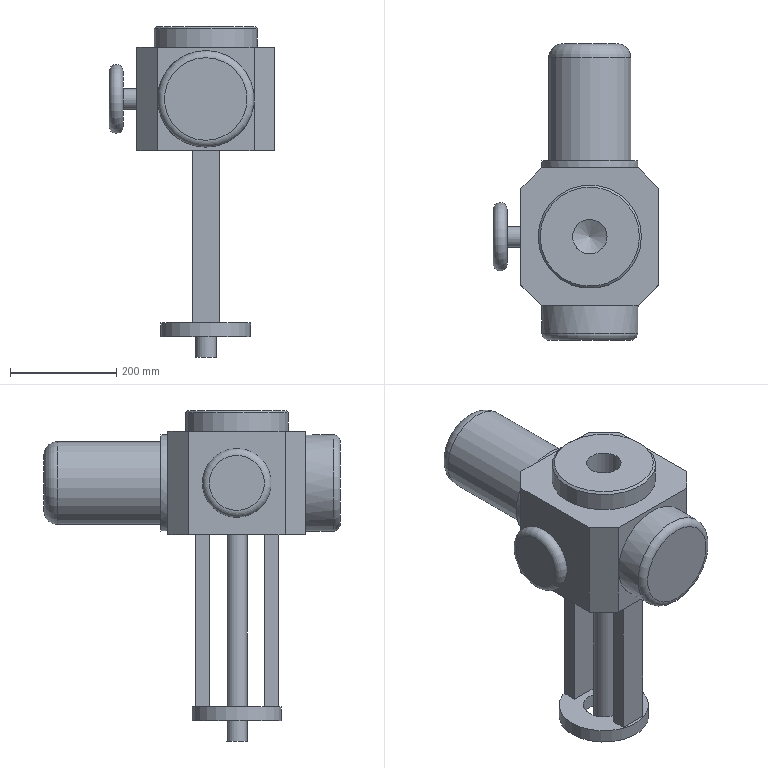Part | NX | features ABSOLUTE_DATUM_PLANE 3, ABSOLUTE_DATUM_AXIS 1, BREP 1 | 1 solid | 49 faces | box 312 x 559 x 624 mm | volume 21569285 mm3 | plane 31 | cylinder 11 | cone 4 | torus 3 | commonest cylinder face diameters 39 x2 182 x2 26 x1 52 x1 65 x1 78 x1
STEP:
#1=CARTESIAN_POINT('',(91.,-130.,578.5));
#2=VERTEX_POINT('',#1);
#3=CARTESIAN_POINT('',(-91.,-130.,578.5));
#4=VERTEX_POINT('',#3);
#5=CARTESIAN_POINT('',(0.,-130.,578.5));
#6=DIRECTION('',(0.,-1.,0.));
#7=DIRECTION('',(0.,0.,-1.));
#8=AXIS2_PLACEMENT_3D('',#5,#6,#7);
#9=CIRCLE('',#8,91.);
#10=EDGE_CURVE('',#2,#4,#9,.T.);
#11=ORIENTED_EDGE('',*,*,#10,.F.);
#12=CARTESIAN_POINT('',(91.,-130.,676.));
#13=VERTEX_POINT('',#12);
#14=CARTESIAN_POINT('',(91.,-130.,481.));
#15=DIRECTION('',(0.,0.,1.));
#16=VECTOR('',#15,1000.);
#17=LINE('',#14,#16);
#18=EDGE_CURVE('',#2,#13,#17,.T.);
#19=ORIENTED_EDGE('',*,*,#18,.T.);
#20=CARTESIAN_POINT('',(-91.,-130.,676.));
#21=VERTEX_POINT('',#20);
#22=CARTESIAN_POINT('',(-130.,-130.,676.));
#23=DIRECTION('',(1.,0.,0.));
#24=VECTOR('',#23,1000.);
#25=LINE('',#22,#24);
#26=EDGE_CURVE('',#21,#13,#25,.T.);
#27=ORIENTED_EDGE('',*,*,#26,.F.);
#28=CARTESIAN_POINT('',(-91.,-130.,481.));
#29=DIRECTION('',(0.,0.,-1.));
#30=VECTOR('',#29,1000.);
#31=LINE('',#28,#30);
#32=EDGE_CURVE('',#21,#4,#31,.T.);
#33=ORIENTED_EDGE('',*,*,#32,.T.);
#34=EDGE_LOOP('',(#11,#19,#27,#33));
#35=FACE_BOUND('',#34,.T.);
#36=CARTESIAN_POINT('',(130.,-130.,481.));
#37=DIRECTION('',(0.,-1.,0.));
#38=DIRECTION('',(0.,0.,-1.));
#39=AXIS2_PLACEMENT_3D('',#36,#37,#38);
#40=PLANE('',#39);
#41=ADVANCED_FACE('',(#35),#40,.T.);
#42=CARTESIAN_POINT('',(91.,130.,578.5));
#43=VERTEX_POINT('',#42);
#44=CARTESIAN_POINT('',(-91.,130.,578.5));
#45=VERTEX_POINT('',#44);
#46=CARTESIAN_POINT('',(0.,130.,578.5));
#47=DIRECTION('',(0.,1.,0.));
#48=DIRECTION('',(0.,0.,1.));
#49=AXIS2_PLACEMENT_3D('',#46,#47,#48);
#50=CIRCLE('',#49,91.);
#51=EDGE_CURVE('',#43,#45,#50,.T.);
#52=ORIENTED_EDGE('',*,*,#51,.F.);
#53=CARTESIAN_POINT('',(91.,130.,481.));
#54=VERTEX_POINT('',#53);
#55=CARTESIAN_POINT('',(91.,130.,481.));
#56=DIRECTION('',(0.,0.,-1.));
#57=VECTOR('',#56,1000.);
#58=LINE('',#55,#57);
#59=EDGE_CURVE('',#43,#54,#58,.T.);
#60=ORIENTED_EDGE('',*,*,#59,.T.);
#61=CARTESIAN_POINT('',(-91.,130.,481.));
#62=VERTEX_POINT('',#61);
#63=CARTESIAN_POINT('',(-130.,130.,481.));
#64=DIRECTION('',(1.,0.,0.));
#65=VECTOR('',#64,1000.);
#66=LINE('',#63,#65);
#67=EDGE_CURVE('',#62,#54,#66,.T.);
#68=ORIENTED_EDGE('',*,*,#67,.F.);
#69=CARTESIAN_POINT('',(-91.,130.,481.));
#70=DIRECTION('',(0.,0.,1.));
#71=VECTOR('',#70,1000.);
#72=LINE('',#69,#71);
#73=EDGE_CURVE('',#62,#45,#72,.T.);
#74=ORIENTED_EDGE('',*,*,#73,.T.);
#75=EDGE_LOOP('',(#52,#60,#68,#74));
#76=FACE_BOUND('',#75,.T.);
#77=CARTESIAN_POINT('',(-130.,130.,481.));
#78=DIRECTION('',(0.,1.,0.));
#79=DIRECTION('',(0.,0.,1.));
#80=AXIS2_PLACEMENT_3D('',#77,#78,#79);
#81=PLANE('',#80);
#82=ADVANCED_FACE('',(#76),#81,.T.);
#83=CARTESIAN_POINT('',(-26.,-78.,156.));
#84=VERTEX_POINT('',#83);
#85=CARTESIAN_POINT('',(-26.,-52.,156.));
#86=VERTEX_POINT('',#85);
#87=CARTESIAN_POINT('',(-26.,-78.,156.));
#88=DIRECTION('',(0.,1.,0.));
#89=VECTOR('',#88,1000.);
#90=LINE('',#87,#89);
#91=EDGE_CURVE('',#84,#86,#90,.T.);
#92=ORIENTED_EDGE('',*,*,#91,.T.);
#93=CARTESIAN_POINT('',(26.,-52.,156.));
#94=VERTEX_POINT('',#93);
#95=CARTESIAN_POINT('',(-26.,-52.,156.));
#96=DIRECTION('',(1.,0.,0.));
#97=VECTOR('',#96,1000.);
#98=LINE('',#95,#97);
#99=EDGE_CURVE('',#86,#94,#98,.T.);
#100=ORIENTED_EDGE('',*,*,#99,.T.);
#101=CARTESIAN_POINT('',(26.,-78.,156.));
#102=VERTEX_POINT('',#101);
#103=CARTESIAN_POINT('',(26.,-78.,156.));
#104=DIRECTION('',(0.,1.,0.));
#105=VECTOR('',#104,1000.);
#106=LINE('',#103,#105);
#107=EDGE_CURVE('',#102,#94,#106,.T.);
#108=ORIENTED_EDGE('',*,*,#107,.F.);
#109=CARTESIAN_POINT('',(-26.,-78.,156.));
#110=DIRECTION('',(1.,0.,0.));
#111=VECTOR('',#110,1000.);
#112=LINE('',#109,#111);
#113=EDGE_CURVE('',#84,#102,#112,.T.);
#114=ORIENTED_EDGE('',*,*,#113,.F.);
#115=EDGE_LOOP('',(#92,#100,#108,#114));
#116=FACE_BOUND('',#115,.T.);
#117=CARTESIAN_POINT('',(-26.,52.,156.));
#118=VERTEX_POINT('',#117);
#119=CARTESIAN_POINT('',(-26.,78.,156.));
#120=VERTEX_POINT('',#119);
#121=CARTESIAN_POINT('',(-26.,52.,156.));
#122=DIRECTION('',(0.,1.,0.));
#123=VECTOR('',#122,1000.);
#124=LINE('',#121,#123);
#125=EDGE_CURVE('',#118,#120,#124,.T.);
#126=ORIENTED_EDGE('',*,*,#125,.T.);
#127=CARTESIAN_POINT('',(26.,78.,156.));
#128=VERTEX_POINT('',#127);
#129=CARTESIAN_POINT('',(-26.,78.,156.));
#130=DIRECTION('',(1.,0.,0.));
#131=VECTOR('',#130,1000.);
#132=LINE('',#129,#131);
#133=EDGE_CURVE('',#120,#128,#132,.T.);
#134=ORIENTED_EDGE('',*,*,#133,.T.);
#135=CARTESIAN_POINT('',(26.,52.,156.));
#136=VERTEX_POINT('',#135);
#137=CARTESIAN_POINT('',(26.,52.,156.));
#138=DIRECTION('',(0.,1.,0.));
#139=VECTOR('',#138,1000.);
#140=LINE('',#137,#139);
#141=EDGE_CURVE('',#136,#128,#140,.T.);
#142=ORIENTED_EDGE('',*,*,#141,.F.);
#143=CARTESIAN_POINT('',(-26.,52.,156.));
#144=DIRECTION('',(1.,0.,0.));
#145=VECTOR('',#144,1000.);
#146=LINE('',#143,#145);
#147=EDGE_CURVE('',#118,#136,#146,.T.);
#148=ORIENTED_EDGE('',*,*,#147,.F.);
#149=EDGE_LOOP('',(#126,#134,#142,#148));
#150=FACE_BOUND('',#149,.T.);
#151=CARTESIAN_POINT('',(39.,0.,156.));
#152=VERTEX_POINT('',#151);
#153=CARTESIAN_POINT('',(0.,0.,156.));
#154=DIRECTION('',(0.,0.,1.));
#155=DIRECTION('',(1.,0.,0.));
#156=AXIS2_PLACEMENT_3D('',#153,#154,#155);
#157=CIRCLE('',#156,39.);
#158=EDGE_CURVE('',#152,#152,#157,.F.);
#159=ORIENTED_EDGE('',*,*,#158,.T.);
#160=EDGE_LOOP('',(#159));
#161=FACE_BOUND('',#160,.T.);
#162=CARTESIAN_POINT('',(-84.5,0.,156.));
#163=VERTEX_POINT('',#162);
#164=CARTESIAN_POINT('',(0.,0.,156.));
#165=DIRECTION('',(0.,0.,-1.));
#166=DIRECTION('',(-1.,0.,0.));
#167=AXIS2_PLACEMENT_3D('',#164,#165,#166);
#168=CIRCLE('',#167,84.5);
#169=EDGE_CURVE('',#163,#163,#168,.T.);
#170=ORIENTED_EDGE('',*,*,#169,.F.);
#171=EDGE_LOOP('',(#170));
#172=FACE_BOUND('',#171,.T.);
#173=CARTESIAN_POINT('',(0.,0.,156.));
#174=DIRECTION('',(0.,0.,1.));
#175=DIRECTION('',(1.,0.,0.));
#176=AXIS2_PLACEMENT_3D('',#173,#174,#175);
#177=PLANE('',#176);
#178=ADVANCED_FACE('',(#116,#150,#161,#172),#177,.T.);
#179=CARTESIAN_POINT('',(39.,0.,130.));
#180=VERTEX_POINT('',#179);
#181=CARTESIAN_POINT('',(0.,0.,130.));
#182=DIRECTION('',(0.,0.,1.));
#183=DIRECTION('',(1.,0.,0.));
#184=AXIS2_PLACEMENT_3D('',#181,#182,#183);
#185=CIRCLE('',#184,39.);
#186=EDGE_CURVE('',#180,#180,#185,.T.);
#187=ORIENTED_EDGE('',*,*,#186,.T.);
#188=EDGE_LOOP('',(#187));
#189=FACE_BOUND('',#188,.T.);
#190=CARTESIAN_POINT('',(84.5,0.,130.));
#191=VERTEX_POINT('',#190);
#192=CARTESIAN_POINT('',(0.,0.,130.));
#193=DIRECTION('',(0.,0.,1.));
#194=DIRECTION('',(1.,0.,0.));
#195=AXIS2_PLACEMENT_3D('',#192,#193,#194);
#196=CIRCLE('',#195,84.5);
#197=EDGE_CURVE('',#191,#191,#196,.T.);
#198=ORIENTED_EDGE('',*,*,#197,.F.);
#199=EDGE_LOOP('',(#198));
#200=FACE_BOUND('',#199,.T.);
#201=CARTESIAN_POINT('',(0.,0.,130.));
#202=DIRECTION('',(0.,0.,-1.));
#203=DIRECTION('',(-1.,0.,0.));
#204=AXIS2_PLACEMENT_3D('',#201,#202,#203);
#205=PLANE('',#204);
#206=ADVANCED_FACE('',(#189,#200),#205,.T.);
#207=ORIENTED_EDGE('',*,*,#169,.T.);
#208=EDGE_LOOP('',(#207));
#209=FACE_BOUND('',#208,.T.);
#210=ORIENTED_EDGE('',*,*,#197,.T.);
#211=EDGE_LOOP('',(#210));
#212=FACE_BOUND('',#211,.T.);
#213=CARTESIAN_POINT('',(0.,0.,130.));
#214=DIRECTION('',(0.,0.,1.));
#215=DIRECTION('',(1.,0.,0.));
#216=AXIS2_PLACEMENT_3D('',#213,#214,#215);
#217=CYLINDRICAL_SURFACE('',#216,84.5);
#218=ADVANCED_FACE('',(#209,#212),#217,.T.);
#219=ORIENTED_EDGE('',*,*,#158,.F.);
#220=EDGE_LOOP('',(#219));
#221=FACE_BOUND('',#220,.T.);
#222=ORIENTED_EDGE('',*,*,#186,.F.);
#223=EDGE_LOOP('',(#222));
#224=FACE_BOUND('',#223,.T.);
#225=CARTESIAN_POINT('',(0.,0.,130.));
#226=DIRECTION('',(0.,0.,1.));
#227=DIRECTION('',(1.,0.,0.));
#228=AXIS2_PLACEMENT_3D('',#225,#226,#227);
#229=CYLINDRICAL_SURFACE('',#228,39.);
#230=ADVANCED_FACE('',(#221,#224),#229,.F.);
#231=ORIENTED_EDGE('',*,*,#125,.F.);
#232=CARTESIAN_POINT('',(-26.,52.,481.));
#233=VERTEX_POINT('',#232);
#234=CARTESIAN_POINT('',(-26.,52.,481.));
#235=DIRECTION('',(0.,0.,1.));
#236=VECTOR('',#235,1000.);
#237=LINE('',#234,#236);
#238=EDGE_CURVE('',#118,#233,#237,.T.);
#239=ORIENTED_EDGE('',*,*,#238,.T.);
#240=CARTESIAN_POINT('',(-26.,78.,481.));
#241=VERTEX_POINT('',#240);
#242=CARTESIAN_POINT('',(-26.,52.,481.));
#243=DIRECTION('',(0.,1.,0.));
#244=VECTOR('',#243,1000.);
#245=LINE('',#242,#244);
#246=EDGE_CURVE('',#233,#241,#245,.T.);
#247=ORIENTED_EDGE('',*,*,#246,.T.);
#248=CARTESIAN_POINT('',(-26.,78.,481.));
#249=DIRECTION('',(0.,0.,1.));
#250=VECTOR('',#249,1000.);
#251=LINE('',#248,#250);
#252=EDGE_CURVE('',#120,#241,#251,.T.);
#253=ORIENTED_EDGE('',*,*,#252,.F.);
#254=EDGE_LOOP('',(#231,#239,#247,#253));
#255=FACE_BOUND('',#254,.T.);
#256=CARTESIAN_POINT('',(-26.,52.,156.));
#257=DIRECTION('',(-1.,0.,0.));
#258=DIRECTION('',(0.,0.,1.));
#259=AXIS2_PLACEMENT_3D('',#256,#257,#258);
#260=PLANE('',#259);
#261=ADVANCED_FACE('',(#255),#260,.T.);
#262=ORIENTED_EDGE('',*,*,#133,.F.);
#263=ORIENTED_EDGE('',*,*,#252,.T.);
#264=CARTESIAN_POINT('',(26.,78.,481.));
#265=VERTEX_POINT('',#264);
#266=CARTESIAN_POINT('',(-26.,78.,481.));
#267=DIRECTION('',(1.,0.,0.));
#268=VECTOR('',#267,1000.);
#269=LINE('',#266,#268);
#270=EDGE_CURVE('',#241,#265,#269,.T.);
#271=ORIENTED_EDGE('',*,*,#270,.T.);
#272=CARTESIAN_POINT('',(26.,78.,481.));
#273=DIRECTION('',(0.,0.,1.));
#274=VECTOR('',#273,1000.);
#275=LINE('',#272,#274);
#276=EDGE_CURVE('',#128,#265,#275,.T.);
#277=ORIENTED_EDGE('',*,*,#276,.F.);
#278=EDGE_LOOP('',(#262,#263,#271,#277));
#279=FACE_BOUND('',#278,.T.);
#280=CARTESIAN_POINT('',(-26.,78.,156.));
#281=DIRECTION('',(0.,1.,0.));
#282=DIRECTION('',(0.,0.,1.));
#283=AXIS2_PLACEMENT_3D('',#280,#281,#282);
#284=PLANE('',#283);
#285=ADVANCED_FACE('',(#279),#284,.T.);
#286=ORIENTED_EDGE('',*,*,#141,.T.);
#287=ORIENTED_EDGE('',*,*,#276,.T.);
#288=CARTESIAN_POINT('',(26.,52.,481.));
#289=VERTEX_POINT('',#288);
#290=CARTESIAN_POINT('',(26.,52.,481.));
#291=DIRECTION('',(0.,1.,0.));
#292=VECTOR('',#291,1000.);
#293=LINE('',#290,#292);
#294=EDGE_CURVE('',#289,#265,#293,.T.);
#295=ORIENTED_EDGE('',*,*,#294,.F.);
#296=CARTESIAN_POINT('',(26.,52.,481.));
#297=DIRECTION('',(0.,0.,1.));
#298=VECTOR('',#297,1000.);
#299=LINE('',#296,#298);
#300=EDGE_CURVE('',#136,#289,#299,.T.);
#301=ORIENTED_EDGE('',*,*,#300,.F.);
#302=EDGE_LOOP('',(#286,#287,#295,#301));
#303=FACE_BOUND('',#302,.T.);
#304=CARTESIAN_POINT('',(26.,78.,156.));
#305=DIRECTION('',(1.,0.,0.));
#306=DIRECTION('',(0.,0.,-1.));
#307=AXIS2_PLACEMENT_3D('',#304,#305,#306);
#308=PLANE('',#307);
#309=ADVANCED_FACE('',(#303),#308,.T.);
#310=ORIENTED_EDGE('',*,*,#238,.F.);
#311=ORIENTED_EDGE('',*,*,#147,.T.);
#312=ORIENTED_EDGE('',*,*,#300,.T.);
#313=CARTESIAN_POINT('',(-26.,52.,481.));
#314=DIRECTION('',(1.,0.,0.));
#315=VECTOR('',#314,1000.);
#316=LINE('',#313,#315);
#317=EDGE_CURVE('',#233,#289,#316,.T.);
#318=ORIENTED_EDGE('',*,*,#317,.F.);
#319=EDGE_LOOP('',(#310,#311,#312,#318));
#320=FACE_BOUND('',#319,.T.);
#321=CARTESIAN_POINT('',(26.,52.,156.));
#322=DIRECTION('',(0.,-1.,0.));
#323=DIRECTION('',(0.,0.,-1.));
#324=AXIS2_PLACEMENT_3D('',#321,#322,#323);
#325=PLANE('',#324);
#326=ADVANCED_FACE('',(#320),#325,.T.);
#327=ORIENTED_EDGE('',*,*,#91,.F.);
#328=CARTESIAN_POINT('',(-26.,-78.,481.));
#329=VERTEX_POINT('',#328);
#330=CARTESIAN_POINT('',(-26.,-78.,481.));
#331=DIRECTION('',(0.,0.,1.));
#332=VECTOR('',#331,1000.);
#333=LINE('',#330,#332);
#334=EDGE_CURVE('',#84,#329,#333,.T.);
#335=ORIENTED_EDGE('',*,*,#334,.T.);
#336=CARTESIAN_POINT('',(-26.,-52.,481.));
#337=VERTEX_POINT('',#336);
#338=CARTESIAN_POINT('',(-26.,-78.,481.));
#339=DIRECTION('',(0.,1.,0.));
#340=VECTOR('',#339,1000.);
#341=LINE('',#338,#340);
#342=EDGE_CURVE('',#329,#337,#341,.T.);
#343=ORIENTED_EDGE('',*,*,#342,.T.);
#344=CARTESIAN_POINT('',(-26.,-52.,481.));
#345=DIRECTION('',(0.,0.,1.));
#346=VECTOR('',#345,1000.);
#347=LINE('',#344,#346);
#348=EDGE_CURVE('',#86,#337,#347,.T.);
#349=ORIENTED_EDGE('',*,*,#348,.F.);
#350=EDGE_LOOP('',(#327,#335,#343,#349));
#351=FACE_BOUND('',#350,.T.);
#352=CARTESIAN_POINT('',(-26.,-78.,156.));
#353=DIRECTION('',(-1.,0.,0.));
#354=DIRECTION('',(0.,0.,1.));
#355=AXIS2_PLACEMENT_3D('',#352,#353,#354);
#356=PLANE('',#355);
#357=ADVANCED_FACE('',(#351),#356,.T.);
#358=ORIENTED_EDGE('',*,*,#99,.F.);
#359=ORIENTED_EDGE('',*,*,#348,.T.);
#360=CARTESIAN_POINT('',(26.,-52.,481.));
#361=VERTEX_POINT('',#360);
#362=CARTESIAN_POINT('',(-26.,-52.,481.));
#363=DIRECTION('',(1.,0.,0.));
#364=VECTOR('',#363,1000.);
#365=LINE('',#362,#364);
#366=EDGE_CURVE('',#337,#361,#365,.T.);
#367=ORIENTED_EDGE('',*,*,#366,.T.);
#368=CARTESIAN_POINT('',(26.,-52.,481.));
#369=DIRECTION('',(0.,0.,1.));
#370=VECTOR('',#369,1000.);
#371=LINE('',#368,#370);
#372=EDGE_CURVE('',#94,#361,#371,.T.);
#373=ORIENTED_EDGE('',*,*,#372,.F.);
#374=EDGE_LOOP('',(#358,#359,#367,#373));
#375=FACE_BOUND('',#374,.T.);
#376=CARTESIAN_POINT('',(-26.,-52.,156.));
#377=DIRECTION('',(0.,1.,0.));
#378=DIRECTION('',(0.,0.,1.));
#379=AXIS2_PLACEMENT_3D('',#376,#377,#378);
#380=PLANE('',#379);
#381=ADVANCED_FACE('',(#375),#380,.T.);
#382=ORIENTED_EDGE('',*,*,#107,.T.);
#383=ORIENTED_EDGE('',*,*,#372,.T.);
#384=CARTESIAN_POINT('',(26.,-78.,481.));
#385=VERTEX_POINT('',#384);
#386=CARTESIAN_POINT('',(26.,-78.,481.));
#387=DIRECTION('',(0.,1.,0.));
#388=VECTOR('',#387,1000.);
#389=LINE('',#386,#388);
#390=EDGE_CURVE('',#385,#361,#389,.T.);
#391=ORIENTED_EDGE('',*,*,#390,.F.);
#392=CARTESIAN_POINT('',(26.,-78.,481.));
#393=DIRECTION('',(0.,0.,1.));
#394=VECTOR('',#393,1000.);
#395=LINE('',#392,#394);
#396=EDGE_CURVE('',#102,#385,#395,.T.);
#397=ORIENTED_EDGE('',*,*,#396,.F.);
#398=EDGE_LOOP('',(#382,#383,#391,#397));
#399=FACE_BOUND('',#398,.T.);
#400=CARTESIAN_POINT('',(26.,-52.,156.));
#401=DIRECTION('',(1.,0.,0.));
#402=DIRECTION('',(0.,0.,-1.));
#403=AXIS2_PLACEMENT_3D('',#400,#401,#402);
#404=PLANE('',#403);
#405=ADVANCED_FACE('',(#399),#404,.T.);
#406=ORIENTED_EDGE('',*,*,#334,.F.);
#407=ORIENTED_EDGE('',*,*,#113,.T.);
#408=ORIENTED_EDGE('',*,*,#396,.T.);
#409=CARTESIAN_POINT('',(-26.,-78.,481.));
#410=DIRECTION('',(1.,0.,0.));
#411=VECTOR('',#410,1000.);
#412=LINE('',#409,#411);
#413=EDGE_CURVE('',#329,#385,#412,.T.);
#414=ORIENTED_EDGE('',*,*,#413,.F.);
#415=EDGE_LOOP('',(#406,#407,#408,#414));
#416=FACE_BOUND('',#415,.T.);
#417=CARTESIAN_POINT('',(26.,-78.,156.));
#418=DIRECTION('',(0.,-1.,0.));
#419=DIRECTION('',(0.,0.,-1.));
#420=AXIS2_PLACEMENT_3D('',#417,#418,#419);
#421=PLANE('',#420);
#422=ADVANCED_FACE('',(#416),#421,.T.);
#423=CARTESIAN_POINT('',(-130.,0.,598.));
#424=VERTEX_POINT('',#423);
#425=CARTESIAN_POINT('',(-130.,0.,578.5));
#426=DIRECTION('',(-1.,0.,0.));
#427=DIRECTION('',(0.,0.,1.));
#428=AXIS2_PLACEMENT_3D('',#425,#426,#427);
#429=CIRCLE('',#428,19.5);
#430=EDGE_CURVE('',#424,#424,#429,.T.);
#431=ORIENTED_EDGE('',*,*,#430,.F.);
#432=EDGE_LOOP('',(#431));
#433=FACE_BOUND('',#432,.T.);
#434=CARTESIAN_POINT('',(-130.,-91.,676.));
#435=VERTEX_POINT('',#434);
#436=CARTESIAN_POINT('',(-130.,91.,676.));
#437=VERTEX_POINT('',#436);
#438=CARTESIAN_POINT('',(-130.,-130.,676.));
#439=DIRECTION('',(0.,1.,0.));
#440=VECTOR('',#439,1000.);
#441=LINE('',#438,#440);
#442=EDGE_CURVE('',#435,#437,#441,.T.);
#443=ORIENTED_EDGE('',*,*,#442,.T.);
#444=CARTESIAN_POINT('',(-130.,91.,481.));
#445=VERTEX_POINT('',#444);
#446=CARTESIAN_POINT('',(-130.,91.,481.));
#447=DIRECTION('',(0.,0.,-1.));
#448=VECTOR('',#447,1000.);
#449=LINE('',#446,#448);
#450=EDGE_CURVE('',#437,#445,#449,.T.);
#451=ORIENTED_EDGE('',*,*,#450,.T.);
#452=CARTESIAN_POINT('',(-130.,-91.,481.));
#453=VERTEX_POINT('',#452);
#454=CARTESIAN_POINT('',(-130.,-130.,481.));
#455=DIRECTION('',(0.,1.,0.));
#456=VECTOR('',#455,1000.);
#457=LINE('',#454,#456);
#458=EDGE_CURVE('',#453,#445,#457,.T.);
#459=ORIENTED_EDGE('',*,*,#458,.F.);
#460=CARTESIAN_POINT('',(-130.,-91.,481.));
#461=DIRECTION('',(0.,0.,1.));
#462=VECTOR('',#461,1000.);
#463=LINE('',#460,#462);
#464=EDGE_CURVE('',#453,#435,#463,.T.);
#465=ORIENTED_EDGE('',*,*,#464,.T.);
#466=EDGE_LOOP('',(#443,#451,#459,#465));
#467=FACE_BOUND('',#466,.T.);
#468=CARTESIAN_POINT('',(-130.,-130.,481.));
#469=DIRECTION('',(-1.,0.,0.));
#470=DIRECTION('',(0.,0.,1.));
#471=AXIS2_PLACEMENT_3D('',#468,#469,#470);
#472=PLANE('',#471);
#473=ADVANCED_FACE('',(#433,#467),#472,.T.);
#474=CARTESIAN_POINT('',(0.,130.,578.5));
#475=DIRECTION('',(0.,1.,0.));
#476=DIRECTION('',(0.,0.,1.));
#477=AXIS2_PLACEMENT_3D('',#474,#475,#476);
#478=CIRCLE('',#477,91.);
#479=EDGE_CURVE('',#45,#43,#478,.T.);
#480=ORIENTED_EDGE('',*,*,#479,.F.);
#481=CARTESIAN_POINT('',(-91.,130.,676.));
#482=VERTEX_POINT('',#481);
#483=CARTESIAN_POINT('',(-91.,130.,481.));
#484=DIRECTION('',(0.,0.,1.));
#485=VECTOR('',#484,1000.);
#486=LINE('',#483,#485);
#487=EDGE_CURVE('',#45,#482,#486,.T.);
#488=ORIENTED_EDGE('',*,*,#487,.T.);
#489=CARTESIAN_POINT('',(91.,130.,676.));
#490=VERTEX_POINT('',#489);
#491=CARTESIAN_POINT('',(-130.,130.,676.));
#492=DIRECTION('',(1.,0.,0.));
#493=VECTOR('',#492,1000.);
#494=LINE('',#491,#493);
#495=EDGE_CURVE('',#482,#490,#494,.T.);
#496=ORIENTED_EDGE('',*,*,#495,.T.);
#497=CARTESIAN_POINT('',(91.,130.,481.));
#498=DIRECTION('',(0.,0.,-1.));
#499=VECTOR('',#498,1000.);
#500=LINE('',#497,#499);
#501=EDGE_CURVE('',#490,#43,#500,.T.);
#502=ORIENTED_EDGE('',*,*,#501,.T.);
#503=EDGE_LOOP('',(#480,#488,#496,#502));
#504=FACE_BOUND('',#503,.T.);
#505=CARTESIAN_POINT('',(-130.,130.,481.));
#506=DIRECTION('',(0.,1.,0.));
#507=DIRECTION('',(0.,0.,1.));
#508=AXIS2_PLACEMENT_3D('',#505,#506,#507);
#509=PLANE('',#508);
#510=ADVANCED_FACE('',(#504),#509,.T.);
#511=CARTESIAN_POINT('',(130.,-91.,481.));
#512=VERTEX_POINT('',#511);
#513=CARTESIAN_POINT('',(130.,91.,481.));
#514=VERTEX_POINT('',#513);
#515=CARTESIAN_POINT('',(130.,-130.,481.));
#516=DIRECTION('',(0.,1.,0.));
#517=VECTOR('',#516,1000.);
#518=LINE('',#515,#517);
#519=EDGE_CURVE('',#512,#514,#518,.T.);
#520=ORIENTED_EDGE('',*,*,#519,.T.);
#521=CARTESIAN_POINT('',(130.,91.,676.));
#522=VERTEX_POINT('',#521);
#523=CARTESIAN_POINT('',(130.,91.,481.));
#524=DIRECTION('',(0.,0.,1.));
#525=VECTOR('',#524,1000.);
#526=LINE('',#523,#525);
#527=EDGE_CURVE('',#514,#522,#526,.T.);
#528=ORIENTED_EDGE('',*,*,#527,.T.);
#529=CARTESIAN_POINT('',(130.,-91.,676.));
#530=VERTEX_POINT('',#529);
#531=CARTESIAN_POINT('',(130.,-130.,676.));
#532=DIRECTION('',(0.,1.,0.));
#533=VECTOR('',#532,1000.);
#534=LINE('',#531,#533);
#535=EDGE_CURVE('',#530,#522,#534,.T.);
#536=ORIENTED_EDGE('',*,*,#535,.F.);
#537=CARTESIAN_POINT('',(130.,-91.,481.));
#538=DIRECTION('',(0.,0.,-1.));
#539=VECTOR('',#538,1000.);
#540=LINE('',#537,#539);
#541=EDGE_CURVE('',#530,#512,#540,.T.);
#542=ORIENTED_EDGE('',*,*,#541,.T.);
#543=EDGE_LOOP('',(#520,#528,#536,#542));
#544=FACE_BOUND('',#543,.T.);
#545=CARTESIAN_POINT('',(130.,130.,481.));
#546=DIRECTION('',(1.,0.,0.));
#547=DIRECTION('',(0.,0.,-1.));
#548=AXIS2_PLACEMENT_3D('',#545,#546,#547);
#549=PLANE('',#548);
#550=ADVANCED_FACE('',(#544),#549,.T.);
#551=CARTESIAN_POINT('',(-19.5,0.,481.));
#552=VERTEX_POINT('',#551);
#553=CARTESIAN_POINT('',(0.,0.,481.));
#554=DIRECTION('',(0.,0.,-1.));
#555=DIRECTION('',(-1.,0.,0.));
#556=AXIS2_PLACEMENT_3D('',#553,#554,#555);
#557=CIRCLE('',#556,19.5);
#558=EDGE_CURVE('',#552,#552,#557,.T.);
#559=ORIENTED_EDGE('',*,*,#558,.F.);
#560=EDGE_LOOP('',(#559));
#561=FACE_BOUND('',#560,.T.);
#562=ORIENTED_EDGE('',*,*,#270,.F.);
#563=ORIENTED_EDGE('',*,*,#246,.F.);
#564=ORIENTED_EDGE('',*,*,#317,.T.);
#565=ORIENTED_EDGE('',*,*,#294,.T.);
#566=EDGE_LOOP('',(#562,#563,#564,#565));
#567=FACE_BOUND('',#566,.T.);
#568=ORIENTED_EDGE('',*,*,#366,.F.);
#569=ORIENTED_EDGE('',*,*,#342,.F.);
#570=ORIENTED_EDGE('',*,*,#413,.T.);
#571=ORIENTED_EDGE('',*,*,#390,.T.);
#572=EDGE_LOOP('',(#568,#569,#570,#571));
#573=FACE_BOUND('',#572,.T.);
#574=ORIENTED_EDGE('',*,*,#67,.T.);
#575=CARTESIAN_POINT('',(240.5,-19.5,481.));
#576=DIRECTION('',(-0.7071,0.7071,0.));
#577=VECTOR('',#576,1000.);
#578=LINE('',#575,#577);
#579=EDGE_CURVE('',#54,#514,#578,.F.);
#580=ORIENTED_EDGE('',*,*,#579,.T.);
#581=ORIENTED_EDGE('',*,*,#519,.F.);
#582=CARTESIAN_POINT('',(91.,-130.,481.));
#583=VERTEX_POINT('',#582);
#584=CARTESIAN_POINT('',(110.5,-110.5,481.));
#585=DIRECTION('',(0.7071,0.7071,0.));
#586=VECTOR('',#585,1000.);
#587=LINE('',#584,#586);
#588=EDGE_CURVE('',#512,#583,#587,.F.);
#589=ORIENTED_EDGE('',*,*,#588,.T.);
#590=CARTESIAN_POINT('',(-91.,-130.,481.));
#591=VERTEX_POINT('',#590);
#592=CARTESIAN_POINT('',(-130.,-130.,481.));
#593=DIRECTION('',(1.,0.,0.));
#594=VECTOR('',#593,1000.);
#595=LINE('',#592,#594);
#596=EDGE_CURVE('',#591,#583,#595,.T.);
#597=ORIENTED_EDGE('',*,*,#596,.F.);
#598=CARTESIAN_POINT('',(19.5,-240.5,481.));
#599=DIRECTION('',(0.7071,-0.7071,0.));
#600=VECTOR('',#599,1000.);
#601=LINE('',#598,#600);
#602=EDGE_CURVE('',#591,#453,#601,.F.);
#603=ORIENTED_EDGE('',*,*,#602,.T.);
#604=ORIENTED_EDGE('',*,*,#458,.T.);
#605=CARTESIAN_POINT('',(-110.5,110.5,481.));
#606=DIRECTION('',(-0.7071,-0.7071,0.));
#607=VECTOR('',#606,1000.);
#608=LINE('',#605,#607);
#609=EDGE_CURVE('',#445,#62,#608,.F.);
#610=ORIENTED_EDGE('',*,*,#609,.T.);
#611=EDGE_LOOP('',(#574,#580,#581,#589,#597,#603,#604,#610));
#612=FACE_BOUND('',#611,.T.);
#613=CARTESIAN_POINT('',(130.,-130.,481.));
#614=DIRECTION('',(0.,0.,-1.));
#615=DIRECTION('',(-1.,0.,0.));
#616=AXIS2_PLACEMENT_3D('',#613,#614,#615);
#617=PLANE('',#616);
#618=ADVANCED_FACE('',(#561,#567,#573,#612),#617,.T.);
#619=CARTESIAN_POINT('',(0.,-130.,578.5));
#620=DIRECTION('',(0.,-1.,0.));
#621=DIRECTION('',(0.,0.,-1.));
#622=AXIS2_PLACEMENT_3D('',#619,#620,#621);
#623=CIRCLE('',#622,91.);
#624=EDGE_CURVE('',#4,#2,#623,.T.);
#625=ORIENTED_EDGE('',*,*,#624,.F.);
#626=CARTESIAN_POINT('',(-91.,-130.,481.));
#627=DIRECTION('',(0.,0.,-1.));
#628=VECTOR('',#627,1000.);
#629=LINE('',#626,#628);
#630=EDGE_CURVE('',#4,#591,#629,.T.);
#631=ORIENTED_EDGE('',*,*,#630,.T.);
#632=ORIENTED_EDGE('',*,*,#596,.T.);
#633=CARTESIAN_POINT('',(91.,-130.,481.));
#634=DIRECTION('',(0.,0.,1.));
#635=VECTOR('',#634,1000.);
#636=LINE('',#633,#635);
#637=EDGE_CURVE('',#583,#2,#636,.T.);
#638=ORIENTED_EDGE('',*,*,#637,.T.);
#639=EDGE_LOOP('',(#625,#631,#632,#638));
#640=FACE_BOUND('',#639,.T.);
#641=CARTESIAN_POINT('',(130.,-130.,481.));
#642=DIRECTION('',(0.,-1.,0.));
#643=DIRECTION('',(0.,0.,-1.));
#644=AXIS2_PLACEMENT_3D('',#641,#642,#643);
#645=PLANE('',#644);
#646=ADVANCED_FACE('',(#640),#645,.T.);
#647=CARTESIAN_POINT('',(97.5,0.,676.));
#648=VERTEX_POINT('',#647);
#649=CARTESIAN_POINT('',(0.,0.,676.));
#650=DIRECTION('',(0.,0.,1.));
#651=DIRECTION('',(1.,0.,0.));
#652=AXIS2_PLACEMENT_3D('',#649,#650,#651);
#653=CIRCLE('',#652,97.5);
#654=EDGE_CURVE('',#648,#648,#653,.T.);
#655=ORIENTED_EDGE('',*,*,#654,.F.);
#656=EDGE_LOOP('',(#655));
#657=FACE_BOUND('',#656,.T.);
#658=ORIENTED_EDGE('',*,*,#535,.T.);
#659=CARTESIAN_POINT('',(110.5,110.5,676.));
#660=DIRECTION('',(0.7071,-0.7071,0.));
#661=VECTOR('',#660,1000.);
#662=LINE('',#659,#661);
#663=EDGE_CURVE('',#522,#490,#662,.F.);
#664=ORIENTED_EDGE('',*,*,#663,.T.);
#665=ORIENTED_EDGE('',*,*,#495,.F.);
#666=CARTESIAN_POINT('',(-240.5,-19.5,676.));
#667=DIRECTION('',(0.7071,0.7071,0.));
#668=VECTOR('',#667,1000.);
#669=LINE('',#666,#668);
#670=EDGE_CURVE('',#482,#437,#669,.F.);
#671=ORIENTED_EDGE('',*,*,#670,.T.);
#672=ORIENTED_EDGE('',*,*,#442,.F.);
#673=CARTESIAN_POINT('',(-110.5,-110.5,676.));
#674=DIRECTION('',(-0.7071,0.7071,0.));
#675=VECTOR('',#674,1000.);
#676=LINE('',#673,#675);
#677=EDGE_CURVE('',#435,#21,#676,.F.);
#678=ORIENTED_EDGE('',*,*,#677,.T.);
#679=ORIENTED_EDGE('',*,*,#26,.T.);
#680=CARTESIAN_POINT('',(-19.5,-240.5,676.));
#681=DIRECTION('',(-0.7071,-0.7071,0.));
#682=VECTOR('',#681,1000.);
#683=LINE('',#680,#682);
#684=EDGE_CURVE('',#13,#530,#683,.F.);
#685=ORIENTED_EDGE('',*,*,#684,.T.);
#686=EDGE_LOOP('',(#658,#664,#665,#671,#672,#678,#679,#685));
#687=FACE_BOUND('',#686,.T.);
#688=CARTESIAN_POINT('',(-130.,-130.,676.));
#689=DIRECTION('',(0.,0.,1.));
#690=DIRECTION('',(1.,0.,0.));
#691=AXIS2_PLACEMENT_3D('',#688,#689,#690);
#692=PLANE('',#691);
#693=ADVANCED_FACE('',(#657,#687),#692,.T.);
#694=ORIENTED_EDGE('',*,*,#579,.F.);
#695=ORIENTED_EDGE('',*,*,#59,.F.);
#696=ORIENTED_EDGE('',*,*,#501,.F.);
#697=ORIENTED_EDGE('',*,*,#663,.F.);
#698=ORIENTED_EDGE('',*,*,#527,.F.);
#699=EDGE_LOOP('',(#694,#695,#696,#697,#698));
#700=FACE_BOUND('',#699,.T.);
#701=CARTESIAN_POINT('',(130.,91.,481.));
#702=DIRECTION('',(-0.7071,-0.7071,0.));
#703=DIRECTION('',(0.7071,-0.7071,0.));
#704=AXIS2_PLACEMENT_3D('',#701,#702,#703);
#705=PLANE('',#704);
#706=ADVANCED_FACE('',(#700),#705,.F.);
#707=ORIENTED_EDGE('',*,*,#609,.F.);
#708=ORIENTED_EDGE('',*,*,#450,.F.);
#709=ORIENTED_EDGE('',*,*,#670,.F.);
#710=ORIENTED_EDGE('',*,*,#487,.F.);
#711=ORIENTED_EDGE('',*,*,#73,.F.);
#712=EDGE_LOOP('',(#707,#708,#709,#710,#711));
#713=FACE_BOUND('',#712,.T.);
#714=CARTESIAN_POINT('',(-91.,130.,481.));
#715=DIRECTION('',(0.7071,-0.7071,0.));
#716=DIRECTION('',(0.7071,0.7071,0.));
#717=AXIS2_PLACEMENT_3D('',#714,#715,#716);
#718=PLANE('',#717);
#719=ADVANCED_FACE('',(#713),#718,.F.);
#720=ORIENTED_EDGE('',*,*,#588,.F.);
#721=ORIENTED_EDGE('',*,*,#541,.F.);
#722=ORIENTED_EDGE('',*,*,#684,.F.);
#723=ORIENTED_EDGE('',*,*,#18,.F.);
#724=ORIENTED_EDGE('',*,*,#637,.F.);
#725=EDGE_LOOP('',(#720,#721,#722,#723,#724));
#726=FACE_BOUND('',#725,.T.);
#727=CARTESIAN_POINT('',(91.,-130.,481.));
#728=DIRECTION('',(-0.7071,0.7071,0.));
#729=DIRECTION('',(-0.7071,-0.7071,0.));
#730=AXIS2_PLACEMENT_3D('',#727,#728,#729);
#731=PLANE('',#730);
#732=ADVANCED_FACE('',(#726),#731,.F.);
#733=ORIENTED_EDGE('',*,*,#602,.F.);
#734=ORIENTED_EDGE('',*,*,#630,.F.);
#735=ORIENTED_EDGE('',*,*,#32,.F.);
#736=ORIENTED_EDGE('',*,*,#677,.F.);
#737=ORIENTED_EDGE('',*,*,#464,.F.);
#738=EDGE_LOOP('',(#733,#734,#735,#736,#737));
#739=FACE_BOUND('',#738,.T.);
#740=CARTESIAN_POINT('',(-130.,-91.,481.));
#741=DIRECTION('',(0.7071,0.7071,0.));
#742=DIRECTION('',(-0.7071,0.7071,0.));
#743=AXIS2_PLACEMENT_3D('',#740,#741,#742);
#744=PLANE('',#743);
#745=ADVANCED_FACE('',(#739),#744,.F.);
#746=CARTESIAN_POINT('',(-32.5,0.,715.));
#747=VERTEX_POINT('',#746);
#748=CARTESIAN_POINT('',(0.,0.,715.));
#749=DIRECTION('',(0.,0.,-1.));
#750=DIRECTION('',(-1.,0.,0.));
#751=AXIS2_PLACEMENT_3D('',#748,#749,#750);
#752=CIRCLE('',#751,32.5);
#753=EDGE_CURVE('',#747,#747,#752,.T.);
#754=ORIENTED_EDGE('',*,*,#753,.T.);
#755=EDGE_LOOP('',(#754));
#756=FACE_BOUND('',#755,.T.);
#757=CARTESIAN_POINT('',(93.6,0.,715.));
#758=VERTEX_POINT('',#757);
#759=CARTESIAN_POINT('',(0.,0.,715.));
#760=DIRECTION('',(0.,0.,1.));
#761=DIRECTION('',(1.,0.,0.));
#762=AXIS2_PLACEMENT_3D('',#759,#760,#761);
#763=CIRCLE('',#762,93.6);
#764=EDGE_CURVE('',#758,#758,#763,.T.);
#765=ORIENTED_EDGE('',*,*,#764,.T.);
#766=EDGE_LOOP('',(#765));
#767=FACE_BOUND('',#766,.T.);
#768=CARTESIAN_POINT('',(0.,0.,715.));
#769=DIRECTION('',(0.,0.,1.));
#770=DIRECTION('',(1.,0.,0.));
#771=AXIS2_PLACEMENT_3D('',#768,#769,#770);
#772=PLANE('',#771);
#773=ADVANCED_FACE('',(#756,#767),#772,.T.);
#774=CARTESIAN_POINT('',(97.5,0.,711.1));
#775=VERTEX_POINT('',#774);
#776=CARTESIAN_POINT('',(0.,0.,711.1));
#777=DIRECTION('',(0.,0.,1.));
#778=DIRECTION('',(1.,0.,0.));
#779=AXIS2_PLACEMENT_3D('',#776,#777,#778);
#780=CIRCLE('',#779,97.5);
#781=EDGE_CURVE('',#775,#775,#780,.F.);
#782=ORIENTED_EDGE('',*,*,#781,.T.);
#783=EDGE_LOOP('',(#782));
#784=FACE_BOUND('',#783,.T.);
#785=ORIENTED_EDGE('',*,*,#654,.T.);
#786=EDGE_LOOP('',(#785));
#787=FACE_BOUND('',#786,.T.);
#788=CARTESIAN_POINT('',(0.,0.,676.));
#789=DIRECTION('',(0.,0.,1.));
#790=DIRECTION('',(1.,0.,0.));
#791=AXIS2_PLACEMENT_3D('',#788,#789,#790);
#792=CYLINDRICAL_SURFACE('',#791,97.5);
#793=ADVANCED_FACE('',(#784,#787),#792,.T.);
#794=CARTESIAN_POINT('',(0.,143.,669.5));
#795=VERTEX_POINT('',#794);
#796=CARTESIAN_POINT('',(0.,143.,578.5));
#797=DIRECTION('',(0.,1.,0.));
#798=DIRECTION('',(0.,0.,1.));
#799=AXIS2_PLACEMENT_3D('',#796,#797,#798);
#800=CIRCLE('',#799,91.);
#801=EDGE_CURVE('',#795,#795,#800,.T.);
#802=ORIENTED_EDGE('',*,*,#801,.T.);
#803=EDGE_LOOP('',(#802));
#804=FACE_BOUND('',#803,.T.);
#805=CARTESIAN_POINT('',(0.,143.,500.5));
#806=VERTEX_POINT('',#805);
#807=CARTESIAN_POINT('',(0.,143.,578.5));
#808=DIRECTION('',(0.,-1.,0.));
#809=DIRECTION('',(0.,0.,-1.));
#810=AXIS2_PLACEMENT_3D('',#807,#808,#809);
#811=CIRCLE('',#810,78.);
#812=EDGE_CURVE('',#806,#806,#811,.T.);
#813=ORIENTED_EDGE('',*,*,#812,.T.);
#814=EDGE_LOOP('',(#813));
#815=FACE_BOUND('',#814,.T.);
#816=CARTESIAN_POINT('',(0.,143.,578.5));
#817=DIRECTION('',(0.,-1.,0.));
#818=DIRECTION('',(0.,0.,-1.));
#819=AXIS2_PLACEMENT_3D('',#816,#817,#818);
#820=PLANE('',#819);
#821=ADVANCED_FACE('',(#804,#815),#820,.F.);
#822=ORIENTED_EDGE('',*,*,#51,.T.);
#823=ORIENTED_EDGE('',*,*,#479,.T.);
#824=EDGE_LOOP('',(#822,#823));
#825=FACE_BOUND('',#824,.T.);
#826=ORIENTED_EDGE('',*,*,#801,.F.);
#827=EDGE_LOOP('',(#826));
#828=FACE_BOUND('',#827,.T.);
#829=CARTESIAN_POINT('',(0.,130.,578.5));
#830=DIRECTION('',(0.,1.,0.));
#831=DIRECTION('',(0.,0.,1.));
#832=AXIS2_PLACEMENT_3D('',#829,#830,#831);
#833=CYLINDRICAL_SURFACE('',#832,91.);
#834=ADVANCED_FACE('',(#825,#828),#833,.T.);
#835=CARTESIAN_POINT('',(0.,364.,630.5));
#836=VERTEX_POINT('',#835);
#837=CARTESIAN_POINT('',(0.,364.,578.5));
#838=DIRECTION('',(0.,1.,0.));
#839=DIRECTION('',(0.,0.,1.));
#840=AXIS2_PLACEMENT_3D('',#837,#838,#839);
#841=CIRCLE('',#840,52.);
#842=EDGE_CURVE('',#836,#836,#841,.T.);
#843=ORIENTED_EDGE('',*,*,#842,.T.);
#844=EDGE_LOOP('',(#843));
#845=FACE_BOUND('',#844,.T.);
#846=CARTESIAN_POINT('',(0.,364.,578.5));
#847=DIRECTION('',(0.,1.,0.));
#848=DIRECTION('',(0.,0.,1.));
#849=AXIS2_PLACEMENT_3D('',#846,#847,#848);
#850=PLANE('',#849);
#851=ADVANCED_FACE('',(#845),#850,.T.);
#852=CARTESIAN_POINT('',(0.,338.,656.5));
#853=VERTEX_POINT('',#852);
#854=CARTESIAN_POINT('',(0.,338.,578.5));
#855=DIRECTION('',(0.,1.,0.));
#856=DIRECTION('',(0.,0.,1.));
#857=AXIS2_PLACEMENT_3D('',#854,#855,#856);
#858=CIRCLE('',#857,78.);
#859=EDGE_CURVE('',#853,#853,#858,.F.);
#860=ORIENTED_EDGE('',*,*,#859,.F.);
#861=EDGE_LOOP('',(#860));
#862=FACE_BOUND('',#861,.T.);
#863=ORIENTED_EDGE('',*,*,#842,.F.);
#864=EDGE_LOOP('',(#863));
#865=FACE_BOUND('',#864,.T.);
#866=CARTESIAN_POINT('',(0.,338.,578.5));
#867=DIRECTION('',(0.,1.,0.));
#868=DIRECTION('',(0.,0.,1.));
#869=AXIS2_PLACEMENT_3D('',#866,#867,#868);
#870=TOROIDAL_SURFACE('',#869,52.,26.);
#871=ADVANCED_FACE('',(#862,#865),#870,.T.);
#872=ORIENTED_EDGE('',*,*,#812,.F.);
#873=EDGE_LOOP('',(#872));
#874=FACE_BOUND('',#873,.T.);
#875=ORIENTED_EDGE('',*,*,#859,.T.);
#876=EDGE_LOOP('',(#875));
#877=FACE_BOUND('',#876,.T.);
#878=CARTESIAN_POINT('',(0.,130.,578.5));
#879=DIRECTION('',(0.,1.,0.));
#880=DIRECTION('',(0.,0.,1.));
#881=AXIS2_PLACEMENT_3D('',#878,#879,#880);
#882=CYLINDRICAL_SURFACE('',#881,78.);
#883=ADVANCED_FACE('',(#874,#877),#882,.T.);
#884=CARTESIAN_POINT('',(0.,-195.,500.5));
#885=VERTEX_POINT('',#884);
#886=CARTESIAN_POINT('',(0.,-195.,578.5));
#887=DIRECTION('',(0.,-1.,0.));
#888=DIRECTION('',(0.,0.,-1.));
#889=AXIS2_PLACEMENT_3D('',#886,#887,#888);
#890=CIRCLE('',#889,78.);
#891=EDGE_CURVE('',#885,#885,#890,.T.);
#892=ORIENTED_EDGE('',*,*,#891,.T.);
#893=EDGE_LOOP('',(#892));
#894=FACE_BOUND('',#893,.T.);
#895=CARTESIAN_POINT('',(0.,-195.,578.5));
#896=DIRECTION('',(0.,-1.,0.));
#897=DIRECTION('',(0.,0.,-1.));
#898=AXIS2_PLACEMENT_3D('',#895,#896,#897);
#899=PLANE('',#898);
#900=ADVANCED_FACE('',(#894),#899,.T.);
#901=CARTESIAN_POINT('',(0.,-182.,487.5));
#902=VERTEX_POINT('',#901);
#903=CARTESIAN_POINT('',(0.,-182.,578.5));
#904=DIRECTION('',(0.,-1.,0.));
#905=DIRECTION('',(0.,0.,-1.));
#906=AXIS2_PLACEMENT_3D('',#903,#904,#905);
#907=CIRCLE('',#906,91.);
#908=EDGE_CURVE('',#902,#902,#907,.F.);
#909=ORIENTED_EDGE('',*,*,#908,.T.);
#910=EDGE_LOOP('',(#909));
#911=FACE_BOUND('',#910,.T.);
#912=ORIENTED_EDGE('',*,*,#10,.T.);
#913=ORIENTED_EDGE('',*,*,#624,.T.);
#914=EDGE_LOOP('',(#912,#913));
#915=FACE_BOUND('',#914,.T.);
#916=CARTESIAN_POINT('',(0.,-130.,578.5));
#917=DIRECTION('',(0.,-1.,0.));
#918=DIRECTION('',(0.,0.,-1.));
#919=AXIS2_PLACEMENT_3D('',#916,#917,#918);
#920=CYLINDRICAL_SURFACE('',#919,91.);
#921=ADVANCED_FACE('',(#911,#915),#920,.T.);
#922=ORIENTED_EDGE('',*,*,#908,.F.);
#923=EDGE_LOOP('',(#922));
#924=FACE_BOUND('',#923,.T.);
#925=ORIENTED_EDGE('',*,*,#891,.F.);
#926=EDGE_LOOP('',(#925));
#927=FACE_BOUND('',#926,.T.);
#928=CARTESIAN_POINT('',(0.,-182.,578.5));
#929=DIRECTION('',(0.,-1.,0.));
#930=DIRECTION('',(0.,0.,-1.));
#931=AXIS2_PLACEMENT_3D('',#928,#929,#930);
#932=TOROIDAL_SURFACE('',#931,78.,13.);
#933=ADVANCED_FACE('',(#924,#927),#932,.T.);
#934=ORIENTED_EDGE('',*,*,#781,.F.);
#935=EDGE_LOOP('',(#934));
#936=FACE_BOUND('',#935,.T.);
#937=ORIENTED_EDGE('',*,*,#764,.F.);
#938=EDGE_LOOP('',(#937));
#939=FACE_BOUND('',#938,.T.);
#940=CARTESIAN_POINT('',(0.,0.,715.));
#941=DIRECTION('',(0.,0.,-1.));
#942=DIRECTION('',(-1.,0.,0.));
#943=AXIS2_PLACEMENT_3D('',#940,#941,#942);
#944=CONICAL_SURFACE('',#943,93.6,0.7854);
#945=ADVANCED_FACE('',(#936,#939),#944,.T.);
#946=CARTESIAN_POINT('',(-156.,0.,598.));
#947=VERTEX_POINT('',#946);
#948=CARTESIAN_POINT('',(-156.,0.,578.5));
#949=DIRECTION('',(-1.,0.,0.));
#950=DIRECTION('',(0.,0.,1.));
#951=AXIS2_PLACEMENT_3D('',#948,#949,#950);
#952=CIRCLE('',#951,19.5);
#953=EDGE_CURVE('',#947,#947,#952,.T.);
#954=ORIENTED_EDGE('',*,*,#953,.F.);
#955=EDGE_LOOP('',(#954));
#956=FACE_BOUND('',#955,.T.);
#957=ORIENTED_EDGE('',*,*,#430,.T.);
#958=EDGE_LOOP('',(#957));
#959=FACE_BOUND('',#958,.T.);
#960=CARTESIAN_POINT('',(-130.,0.,578.5));
#961=DIRECTION('',(-1.,0.,0.));
#962=DIRECTION('',(0.,0.,1.));
#963=AXIS2_PLACEMENT_3D('',#960,#961,#962);
#964=CYLINDRICAL_SURFACE('',#963,19.5);
#965=ADVANCED_FACE('',(#956,#959),#964,.T.);
#966=CARTESIAN_POINT('',(-182.,0.,630.5));
#967=VERTEX_POINT('',#966);
#968=CARTESIAN_POINT('',(-182.,0.,578.5));
#969=DIRECTION('',(-1.,0.,0.));
#970=DIRECTION('',(0.,0.,1.));
#971=AXIS2_PLACEMENT_3D('',#968,#969,#970);
#972=CIRCLE('',#971,52.);
#973=EDGE_CURVE('',#967,#967,#972,.T.);
#974=ORIENTED_EDGE('',*,*,#973,.T.);
#975=EDGE_LOOP('',(#974));
#976=FACE_BOUND('',#975,.T.);
#977=CARTESIAN_POINT('',(-182.,0.,578.5));
#978=DIRECTION('',(-1.,0.,0.));
#979=DIRECTION('',(0.,0.,1.));
#980=AXIS2_PLACEMENT_3D('',#977,#978,#979);
#981=PLANE('',#980);
#982=ADVANCED_FACE('',(#976),#981,.T.);
#983=CARTESIAN_POINT('',(-156.,0.,526.5));
#984=VERTEX_POINT('',#983);
#985=CARTESIAN_POINT('',(-156.,0.,578.5));
#986=DIRECTION('',(1.,0.,0.));
#987=DIRECTION('',(0.,0.,-1.));
#988=AXIS2_PLACEMENT_3D('',#985,#986,#987);
#989=CIRCLE('',#988,52.);
#990=EDGE_CURVE('',#984,#984,#989,.T.);
#991=ORIENTED_EDGE('',*,*,#990,.T.);
#992=EDGE_LOOP('',(#991));
#993=FACE_BOUND('',#992,.T.);
#994=ORIENTED_EDGE('',*,*,#953,.T.);
#995=EDGE_LOOP('',(#994));
#996=FACE_BOUND('',#995,.T.);
#997=CARTESIAN_POINT('',(-156.,0.,578.5));
#998=DIRECTION('',(1.,0.,0.));
#999=DIRECTION('',(0.,0.,-1.));
#1000=AXIS2_PLACEMENT_3D('',#997,#998,#999);
#1001=PLANE('',#1000);
#1002=ADVANCED_FACE('',(#993,#996),#1001,.T.);
#1003=ORIENTED_EDGE('',*,*,#973,.F.);
#1004=EDGE_LOOP('',(#1003));
#1005=FACE_BOUND('',#1004,.T.);
#1006=ORIENTED_EDGE('',*,*,#990,.F.);
#1007=EDGE_LOOP('',(#1006));
#1008=FACE_BOUND('',#1007,.T.);
#1009=CARTESIAN_POINT('',(-169.,0.,578.5));
#1010=DIRECTION('',(-1.,0.,0.));
#1011=DIRECTION('',(0.,0.,1.));
#1012=AXIS2_PLACEMENT_3D('',#1009,#1010,#1011);
#1013=TOROIDAL_SURFACE('',#1012,52.,13.);
#1014=ADVANCED_FACE('',(#1005,#1008),#1013,.T.);
#1015=CARTESIAN_POINT('',(-19.5,0.,91.));
#1016=VERTEX_POINT('',#1015);
#1017=CARTESIAN_POINT('',(0.,0.,91.));
#1018=DIRECTION('',(0.,0.,-1.));
#1019=DIRECTION('',(-1.,0.,0.));
#1020=AXIS2_PLACEMENT_3D('',#1017,#1018,#1019);
#1021=CIRCLE('',#1020,19.5);
#1022=EDGE_CURVE('',#1016,#1016,#1021,.T.);
#1023=ORIENTED_EDGE('',*,*,#1022,.T.);
#1024=EDGE_LOOP('',(#1023));
#1025=FACE_BOUND('',#1024,.T.);
#1026=CARTESIAN_POINT('',(0.,0.,91.));
#1027=DIRECTION('',(0.,0.,-1.));
#1028=DIRECTION('',(-1.,0.,0.));
#1029=AXIS2_PLACEMENT_3D('',#1026,#1027,#1028);
#1030=PLANE('',#1029);
#1031=ADVANCED_FACE('',(#1025),#1030,.T.);
#1032=ORIENTED_EDGE('',*,*,#1022,.F.);
#1033=EDGE_LOOP('',(#1032));
#1034=FACE_BOUND('',#1033,.T.);
#1035=ORIENTED_EDGE('',*,*,#558,.T.);
#1036=EDGE_LOOP('',(#1035));
#1037=FACE_BOUND('',#1036,.T.);
#1038=CARTESIAN_POINT('',(0.,0.,481.));
#1039=DIRECTION('',(0.,0.,-1.));
#1040=DIRECTION('',(-1.,0.,0.));
#1041=AXIS2_PLACEMENT_3D('',#1038,#1039,#1040);
#1042=CYLINDRICAL_SURFACE('',#1041,19.5);
#1043=ADVANCED_FACE('',(#1034,#1037),#1042,.T.);
#1044=CARTESIAN_POINT('',(-32.5,0.,637.));
#1045=VERTEX_POINT('',#1044);
#1046=CARTESIAN_POINT('',(0.,0.,637.));
#1047=DIRECTION('',(0.,0.,-1.));
#1048=DIRECTION('',(-1.,0.,0.));
#1049=AXIS2_PLACEMENT_3D('',#1046,#1047,#1048);
#1050=CIRCLE('',#1049,32.5);
#1051=EDGE_CURVE('',#1045,#1045,#1050,.F.);
#1052=ORIENTED_EDGE('',*,*,#1051,.T.);
#1053=EDGE_LOOP('',(#1052));
#1054=FACE_BOUND('',#1053,.T.);
#1055=CARTESIAN_POINT('',(0.,0.,618.236));
#1056=VERTEX_POINT('',#1055);
#1057=VERTEX_LOOP('',#1056);
#1058=FACE_BOUND('',#1057,.T.);
#1059=CARTESIAN_POINT('',(0.,0.,637.));
#1060=DIRECTION('',(0.,0.,1.));
#1061=DIRECTION('',(1.,0.,0.));
#1062=AXIS2_PLACEMENT_3D('',#1059,#1060,#1061);
#1063=CONICAL_SURFACE('',#1062,32.5,1.047);
#1064=ADVANCED_FACE('',(#1054,#1058),#1063,.F.);
#1065=ORIENTED_EDGE('',*,*,#1051,.F.);
#1066=EDGE_LOOP('',(#1065));
#1067=FACE_BOUND('',#1066,.T.);
#1068=ORIENTED_EDGE('',*,*,#753,.F.);
#1069=EDGE_LOOP('',(#1068));
#1070=FACE_BOUND('',#1069,.T.);
#1071=CARTESIAN_POINT('',(0.,0.,715.));
#1072=DIRECTION('',(0.,0.,-1.));
#1073=DIRECTION('',(-1.,0.,0.));
#1074=AXIS2_PLACEMENT_3D('',#1071,#1072,#1073);
#1075=CYLINDRICAL_SURFACE('',#1074,32.5);
#1076=ADVANCED_FACE('',(#1067,#1070),#1075,.F.);
#1077=CLOSED_SHELL('',(#41,#82,#178,#206,#218,#230,#261,#285,#309,#326,#357,#381,#405,#422,#473,#510,#550,#618,#646,#693,#706,#719,#732,#745,#773,#793,#821,#834,#851,#871,#883,#900,#921,#933,#945,#965,#982,#1002,#1014,#1031,#1043,#1064,#1076));
#1078=CARTESIAN_POINT('',(-130.,0.,565.5));
#1079=VERTEX_POINT('',#1078);
#1080=CARTESIAN_POINT('',(-130.,0.,578.5));
#1081=DIRECTION('',(1.,0.,0.));
#1082=DIRECTION('',(0.,0.,-1.));
#1083=AXIS2_PLACEMENT_3D('',#1080,#1081,#1082);
#1084=CIRCLE('',#1083,13.);
#1085=EDGE_CURVE('',#1079,#1079,#1084,.T.);
#1086=ORIENTED_EDGE('',*,*,#1085,.T.);
#1087=EDGE_LOOP('',(#1086));
#1088=FACE_BOUND('',#1087,.T.);
#1089=CARTESIAN_POINT('',(-130.,0.,578.5));
#1090=DIRECTION('',(1.,0.,0.));
#1091=DIRECTION('',(0.,0.,-1.));
#1092=AXIS2_PLACEMENT_3D('',#1089,#1090,#1091);
#1093=PLANE('',#1092);
#1094=ADVANCED_FACE('',(#1088),#1093,.T.);
#1095=CARTESIAN_POINT('',(-52.,0.,565.5));
#1096=VERTEX_POINT('',#1095);
#1097=CARTESIAN_POINT('',(-52.,0.,578.5));
#1098=DIRECTION('',(1.,0.,0.));
#1099=DIRECTION('',(0.,0.,-1.));
#1100=AXIS2_PLACEMENT_3D('',#1097,#1098,#1099);
#1101=CIRCLE('',#1100,13.);
#1102=EDGE_CURVE('',#1096,#1096,#1101,.F.);
#1103=ORIENTED_EDGE('',*,*,#1102,.T.);
#1104=EDGE_LOOP('',(#1103));
#1105=FACE_BOUND('',#1104,.T.);
#1106=CARTESIAN_POINT('',(-44.494,0.,578.5));
#1107=VERTEX_POINT('',#1106);
#1108=VERTEX_LOOP('',#1107);
#1109=FACE_BOUND('',#1108,.T.);
#1110=CARTESIAN_POINT('',(-52.,0.,578.5));
#1111=DIRECTION('',(-1.,0.,0.));
#1112=DIRECTION('',(0.,0.,1.));
#1113=AXIS2_PLACEMENT_3D('',#1110,#1111,#1112);
#1114=CONICAL_SURFACE('',#1113,13.,1.047);
#1115=ADVANCED_FACE('',(#1105,#1109),#1114,.F.);
#1116=ORIENTED_EDGE('',*,*,#1102,.F.);
#1117=EDGE_LOOP('',(#1116));
#1118=FACE_BOUND('',#1117,.T.);
#1119=ORIENTED_EDGE('',*,*,#1085,.F.);
#1120=EDGE_LOOP('',(#1119));
#1121=FACE_BOUND('',#1120,.T.);
#1122=CARTESIAN_POINT('',(-130.,0.,578.5));
#1123=DIRECTION('',(1.,0.,0.));
#1124=DIRECTION('',(0.,0.,-1.));
#1125=AXIS2_PLACEMENT_3D('',#1122,#1123,#1124);
#1126=CYLINDRICAL_SURFACE('',#1125,13.);
#1127=ADVANCED_FACE('',(#1118,#1121),#1126,.F.);
#1128=CLOSED_SHELL('',(#1094,#1115,#1127));
#1129=ORIENTED_CLOSED_SHELL('',*,#1128,.F.);
#1130=CARTESIAN_POINT('',(0.,130.,552.5));
#1131=VERTEX_POINT('',#1130);
#1132=CARTESIAN_POINT('',(0.,130.,578.5));
#1133=DIRECTION('',(0.,-1.,0.));
#1134=DIRECTION('',(0.,0.,-1.));
#1135=AXIS2_PLACEMENT_3D('',#1132,#1133,#1134);
#1136=CIRCLE('',#1135,26.);
#1137=EDGE_CURVE('',#1131,#1131,#1136,.T.);
#1138=ORIENTED_EDGE('',*,*,#1137,.T.);
#1139=EDGE_LOOP('',(#1138));
#1140=FACE_BOUND('',#1139,.T.);
#1141=CARTESIAN_POINT('',(0.,130.,578.5));
#1142=DIRECTION('',(0.,-1.,0.));
#1143=DIRECTION('',(0.,0.,-1.));
#1144=AXIS2_PLACEMENT_3D('',#1141,#1142,#1143);
#1145=PLANE('',#1144);
#1146=ADVANCED_FACE('',(#1140),#1145,.T.);
#1147=CARTESIAN_POINT('',(0.,52.,552.5));
#1148=VERTEX_POINT('',#1147);
#1149=CARTESIAN_POINT('',(0.,52.,578.5));
#1150=DIRECTION('',(0.,-1.,0.));
#1151=DIRECTION('',(0.,0.,-1.));
#1152=AXIS2_PLACEMENT_3D('',#1149,#1150,#1151);
#1153=CIRCLE('',#1152,26.);
#1154=EDGE_CURVE('',#1148,#1148,#1153,.F.);
#1155=ORIENTED_EDGE('',*,*,#1154,.T.);
#1156=EDGE_LOOP('',(#1155));
#1157=FACE_BOUND('',#1156,.T.);
#1158=CARTESIAN_POINT('',(0.,36.989,578.5));
#1159=VERTEX_POINT('',#1158);
#1160=VERTEX_LOOP('',#1159);
#1161=FACE_BOUND('',#1160,.T.);
#1162=CARTESIAN_POINT('',(0.,52.,578.5));
#1163=DIRECTION('',(0.,1.,0.));
#1164=DIRECTION('',(0.,0.,1.));
#1165=AXIS2_PLACEMENT_3D('',#1162,#1163,#1164);
#1166=CONICAL_SURFACE('',#1165,26.,1.047);
#1167=ADVANCED_FACE('',(#1157,#1161),#1166,.F.);
#1168=ORIENTED_EDGE('',*,*,#1154,.F.);
#1169=EDGE_LOOP('',(#1168));
#1170=FACE_BOUND('',#1169,.T.);
#1171=ORIENTED_EDGE('',*,*,#1137,.F.);
#1172=EDGE_LOOP('',(#1171));
#1173=FACE_BOUND('',#1172,.T.);
#1174=CARTESIAN_POINT('',(0.,130.,578.5));
#1175=DIRECTION('',(0.,-1.,0.));
#1176=DIRECTION('',(0.,0.,-1.));
#1177=AXIS2_PLACEMENT_3D('',#1174,#1175,#1176);
#1178=CYLINDRICAL_SURFACE('',#1177,26.);
#1179=ADVANCED_FACE('',(#1170,#1173),#1178,.F.);
#1180=CLOSED_SHELL('',(#1146,#1167,#1179));
#1181=ORIENTED_CLOSED_SHELL('',*,#1180,.F.);
#1182=BREP_WITH_VOIDS('',#1077,(#1129,#1181));
#1183=(LENGTH_UNIT()NAMED_UNIT(*)SI_UNIT(.MILLI.,.METRE.));
#1184=UNCERTAINTY_MEASURE_WITH_UNIT(LENGTH_MEASURE(0.00001),#1183,'','');
#1185=(NAMED_UNIT(*)PLANE_ANGLE_UNIT()SI_UNIT($,.RADIAN.));
#1186=(NAMED_UNIT(*)SI_UNIT($,.STERADIAN.)SOLID_ANGLE_UNIT());
#1187=(GEOMETRIC_REPRESENTATION_CONTEXT(3)GLOBAL_UNCERTAINTY_ASSIGNED_CONTEXT((#1184))GLOBAL_UNIT_ASSIGNED_CONTEXT((#1183,#1185,#1186))REPRESENTATION_CONTEXT('',''));
#1188=ADVANCED_BREP_SHAPE_REPRESENTATION('',(#1182),#1187);